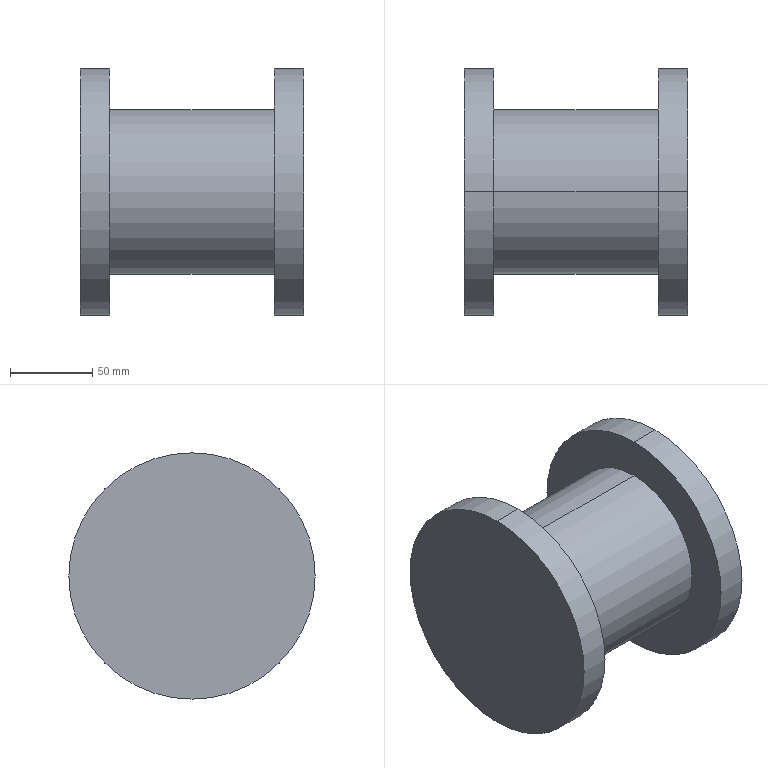Part | SolidWorks | features ICE 2, Extrusion 1 | 1 solid | 10 faces | box 136 x 150 x 150 mm | volume 1421571 mm3 | cylinder 6 | plane 4 | commonest cylinder face diameters 150 x4 100 x2
STEP:
#1=CARTESIAN_POINT('',(-118.,0.,-75.));
#2=VERTEX_POINT('',#1);
#3=CARTESIAN_POINT('',(-118.,0.,75.));
#4=VERTEX_POINT('',#3);
#5=CARTESIAN_POINT('',(-118.,0.,0.));
#6=DIRECTION('',(1.,0.,0.));
#7=DIRECTION('',(0.,0.,-1.));
#8=AXIS2_PLACEMENT_3D('',#5,#6,#7);
#9=CIRCLE('',#8,75.);
#10=EDGE_CURVE('',#2,#4,#9,.T.);
#11=ORIENTED_EDGE('',*,*,#10,.T.);
#12=CARTESIAN_POINT('',(-100.,0.,75.));
#13=VERTEX_POINT('',#12);
#14=CARTESIAN_POINT('',(-118.,0.,75.));
#15=DIRECTION('',(1.,0.,0.));
#16=VECTOR('',#15,1000.);
#17=LINE('',#14,#16);
#18=EDGE_CURVE('',#4,#13,#17,.T.);
#19=ORIENTED_EDGE('',*,*,#18,.T.);
#20=CARTESIAN_POINT('',(-100.,0.,-75.));
#21=VERTEX_POINT('',#20);
#22=CARTESIAN_POINT('',(-100.,0.,0.));
#23=DIRECTION('',(1.,0.,0.));
#24=DIRECTION('',(0.,0.,-1.));
#25=AXIS2_PLACEMENT_3D('',#22,#23,#24);
#26=CIRCLE('',#25,75.);
#27=EDGE_CURVE('',#21,#13,#26,.T.);
#28=ORIENTED_EDGE('',*,*,#27,.F.);
#29=CARTESIAN_POINT('',(-118.,0.,-75.));
#30=DIRECTION('',(1.,0.,0.));
#31=VECTOR('',#30,1000.);
#32=LINE('',#29,#31);
#33=EDGE_CURVE('',#2,#21,#32,.T.);
#34=ORIENTED_EDGE('',*,*,#33,.F.);
#35=EDGE_LOOP('',(#11,#19,#28,#34));
#36=FACE_OUTER_BOUND('',#35,.T.);
#37=CARTESIAN_POINT('',(-118.,0.,0.));
#38=DIRECTION('',(1.,0.,0.));
#39=DIRECTION('',(0.,0.,-1.));
#40=AXIS2_PLACEMENT_3D('',#37,#38,#39);
#41=CYLINDRICAL_SURFACE('',#40,75.);
#42=ADVANCED_FACE('',(#36),#41,.T.);
#43=CARTESIAN_POINT('',(-100.,0.,-50.));
#44=VERTEX_POINT('',#43);
#45=CARTESIAN_POINT('',(-100.,0.,50.));
#46=VERTEX_POINT('',#45);
#47=CARTESIAN_POINT('',(-100.,0.,0.));
#48=DIRECTION('',(1.,0.,0.));
#49=DIRECTION('',(0.,0.,-1.));
#50=AXIS2_PLACEMENT_3D('',#47,#48,#49);
#51=CIRCLE('',#50,50.);
#52=EDGE_CURVE('',#44,#46,#51,.T.);
#53=ORIENTED_EDGE('',*,*,#52,.T.);
#54=CARTESIAN_POINT('',(0.,0.,50.));
#55=VERTEX_POINT('',#54);
#56=CARTESIAN_POINT('',(-100.,0.,50.));
#57=DIRECTION('',(1.,0.,0.));
#58=VECTOR('',#57,1000.);
#59=LINE('',#56,#58);
#60=EDGE_CURVE('',#46,#55,#59,.T.);
#61=ORIENTED_EDGE('',*,*,#60,.T.);
#62=CARTESIAN_POINT('',(0.,0.,-50.));
#63=VERTEX_POINT('',#62);
#64=CARTESIAN_POINT('',(0.,0.,0.));
#65=DIRECTION('',(1.,0.,0.));
#66=DIRECTION('',(0.,0.,-1.));
#67=AXIS2_PLACEMENT_3D('',#64,#65,#66);
#68=CIRCLE('',#67,50.);
#69=EDGE_CURVE('',#63,#55,#68,.T.);
#70=ORIENTED_EDGE('',*,*,#69,.F.);
#71=CARTESIAN_POINT('',(-100.,0.,-50.));
#72=DIRECTION('',(1.,0.,0.));
#73=VECTOR('',#72,1000.);
#74=LINE('',#71,#73);
#75=EDGE_CURVE('',#44,#63,#74,.T.);
#76=ORIENTED_EDGE('',*,*,#75,.F.);
#77=EDGE_LOOP('',(#53,#61,#70,#76));
#78=FACE_OUTER_BOUND('',#77,.T.);
#79=CARTESIAN_POINT('',(-100.,0.,0.));
#80=DIRECTION('',(1.,0.,0.));
#81=DIRECTION('',(0.,0.,-1.));
#82=AXIS2_PLACEMENT_3D('',#79,#80,#81);
#83=CYLINDRICAL_SURFACE('',#82,50.);
#84=ADVANCED_FACE('',(#78),#83,.T.);
#85=CARTESIAN_POINT('',(18.,0.,-75.));
#86=VERTEX_POINT('',#85);
#87=CARTESIAN_POINT('',(18.,0.,75.));
#88=VERTEX_POINT('',#87);
#89=CARTESIAN_POINT('',(18.,0.,0.));
#90=DIRECTION('',(1.,0.,0.));
#91=DIRECTION('',(0.,0.,-1.));
#92=AXIS2_PLACEMENT_3D('',#89,#90,#91);
#93=CIRCLE('',#92,75.);
#94=EDGE_CURVE('',#86,#88,#93,.T.);
#95=ORIENTED_EDGE('',*,*,#94,.F.);
#96=CARTESIAN_POINT('',(0.,0.,-75.));
#97=VERTEX_POINT('',#96);
#98=CARTESIAN_POINT('',(18.,0.,-75.));
#99=DIRECTION('',(-1.,0.,0.));
#100=VECTOR('',#99,1000.);
#101=LINE('',#98,#100);
#102=EDGE_CURVE('',#86,#97,#101,.T.);
#103=ORIENTED_EDGE('',*,*,#102,.T.);
#104=CARTESIAN_POINT('',(0.,0.,75.));
#105=VERTEX_POINT('',#104);
#106=CARTESIAN_POINT('',(0.,0.,0.));
#107=DIRECTION('',(1.,0.,0.));
#108=DIRECTION('',(0.,0.,-1.));
#109=AXIS2_PLACEMENT_3D('',#106,#107,#108);
#110=CIRCLE('',#109,75.);
#111=EDGE_CURVE('',#97,#105,#110,.T.);
#112=ORIENTED_EDGE('',*,*,#111,.T.);
#113=CARTESIAN_POINT('',(18.,0.,75.));
#114=DIRECTION('',(-1.,0.,0.));
#115=VECTOR('',#114,1000.);
#116=LINE('',#113,#115);
#117=EDGE_CURVE('',#88,#105,#116,.T.);
#118=ORIENTED_EDGE('',*,*,#117,.F.);
#119=EDGE_LOOP('',(#95,#103,#112,#118));
#120=FACE_OUTER_BOUND('',#119,.T.);
#121=CARTESIAN_POINT('',(18.,0.,0.));
#122=DIRECTION('',(-1.,0.,0.));
#123=DIRECTION('',(0.,0.,1.));
#124=AXIS2_PLACEMENT_3D('',#121,#122,#123);
#125=CYLINDRICAL_SURFACE('',#124,75.);
#126=ADVANCED_FACE('',(#120),#125,.T.);
#127=ORIENTED_EDGE('',*,*,#102,.F.);
#128=CARTESIAN_POINT('',(18.,0.,0.));
#129=DIRECTION('',(1.,0.,0.));
#130=DIRECTION('',(0.,0.,-1.));
#131=AXIS2_PLACEMENT_3D('',#128,#129,#130);
#132=CIRCLE('',#131,75.);
#133=EDGE_CURVE('',#88,#86,#132,.T.);
#134=ORIENTED_EDGE('',*,*,#133,.F.);
#135=ORIENTED_EDGE('',*,*,#117,.T.);
#136=CARTESIAN_POINT('',(0.,0.,0.));
#137=DIRECTION('',(1.,0.,0.));
#138=DIRECTION('',(0.,0.,-1.));
#139=AXIS2_PLACEMENT_3D('',#136,#137,#138);
#140=CIRCLE('',#139,75.);
#141=EDGE_CURVE('',#105,#97,#140,.T.);
#142=ORIENTED_EDGE('',*,*,#141,.T.);
#143=EDGE_LOOP('',(#127,#134,#135,#142));
#144=FACE_OUTER_BOUND('',#143,.T.);
#145=CARTESIAN_POINT('',(18.,0.,0.));
#146=DIRECTION('',(-1.,0.,0.));
#147=DIRECTION('',(0.,0.,1.));
#148=AXIS2_PLACEMENT_3D('',#145,#146,#147);
#149=CYLINDRICAL_SURFACE('',#148,75.);
#150=ADVANCED_FACE('',(#144),#149,.T.);
#151=ORIENTED_EDGE('',*,*,#69,.T.);
#152=CARTESIAN_POINT('',(0.,0.,0.));
#153=DIRECTION('',(1.,0.,0.));
#154=DIRECTION('',(0.,0.,-1.));
#155=AXIS2_PLACEMENT_3D('',#152,#153,#154);
#156=CIRCLE('',#155,50.);
#157=EDGE_CURVE('',#55,#63,#156,.T.);
#158=ORIENTED_EDGE('',*,*,#157,.T.);
#159=EDGE_LOOP('',(#151,#158));
#160=FACE_BOUND('',#159,.T.);
#161=ORIENTED_EDGE('',*,*,#141,.F.);
#162=ORIENTED_EDGE('',*,*,#111,.F.);
#163=EDGE_LOOP('',(#161,#162));
#164=FACE_OUTER_BOUND('',#163,.T.);
#165=CARTESIAN_POINT('',(0.,0.,0.));
#166=DIRECTION('',(1.,0.,0.));
#167=DIRECTION('',(0.,0.,-1.));
#168=AXIS2_PLACEMENT_3D('',#165,#166,#167);
#169=PLANE('',#168);
#170=ADVANCED_FACE('',(#160,#164),#169,.F.);
#171=ORIENTED_EDGE('',*,*,#133,.T.);
#172=ORIENTED_EDGE('',*,*,#94,.T.);
#173=EDGE_LOOP('',(#171,#172));
#174=FACE_OUTER_BOUND('',#173,.T.);
#175=CARTESIAN_POINT('',(18.,0.,0.));
#176=DIRECTION('',(1.,0.,0.));
#177=DIRECTION('',(0.,0.,-1.));
#178=AXIS2_PLACEMENT_3D('',#175,#176,#177);
#179=PLANE('',#178);
#180=ADVANCED_FACE('',(#174),#179,.T.);
#181=ORIENTED_EDGE('',*,*,#60,.F.);
#182=CARTESIAN_POINT('',(-100.,0.,0.));
#183=DIRECTION('',(1.,0.,0.));
#184=DIRECTION('',(0.,0.,-1.));
#185=AXIS2_PLACEMENT_3D('',#182,#183,#184);
#186=CIRCLE('',#185,50.);
#187=EDGE_CURVE('',#46,#44,#186,.T.);
#188=ORIENTED_EDGE('',*,*,#187,.T.);
#189=ORIENTED_EDGE('',*,*,#75,.T.);
#190=ORIENTED_EDGE('',*,*,#157,.F.);
#191=EDGE_LOOP('',(#181,#188,#189,#190));
#192=FACE_OUTER_BOUND('',#191,.T.);
#193=CARTESIAN_POINT('',(-100.,0.,0.));
#194=DIRECTION('',(1.,0.,0.));
#195=DIRECTION('',(0.,0.,-1.));
#196=AXIS2_PLACEMENT_3D('',#193,#194,#195);
#197=CYLINDRICAL_SURFACE('',#196,50.);
#198=ADVANCED_FACE('',(#192),#197,.T.);
#199=ORIENTED_EDGE('',*,*,#18,.F.);
#200=CARTESIAN_POINT('',(-118.,0.,0.));
#201=DIRECTION('',(1.,0.,0.));
#202=DIRECTION('',(0.,0.,-1.));
#203=AXIS2_PLACEMENT_3D('',#200,#201,#202);
#204=CIRCLE('',#203,75.);
#205=EDGE_CURVE('',#4,#2,#204,.T.);
#206=ORIENTED_EDGE('',*,*,#205,.T.);
#207=ORIENTED_EDGE('',*,*,#33,.T.);
#208=CARTESIAN_POINT('',(-100.,0.,0.));
#209=DIRECTION('',(1.,0.,0.));
#210=DIRECTION('',(0.,0.,-1.));
#211=AXIS2_PLACEMENT_3D('',#208,#209,#210);
#212=CIRCLE('',#211,75.);
#213=EDGE_CURVE('',#13,#21,#212,.T.);
#214=ORIENTED_EDGE('',*,*,#213,.F.);
#215=EDGE_LOOP('',(#199,#206,#207,#214));
#216=FACE_OUTER_BOUND('',#215,.T.);
#217=CARTESIAN_POINT('',(-118.,0.,0.));
#218=DIRECTION('',(1.,0.,0.));
#219=DIRECTION('',(0.,0.,-1.));
#220=AXIS2_PLACEMENT_3D('',#217,#218,#219);
#221=CYLINDRICAL_SURFACE('',#220,75.);
#222=ADVANCED_FACE('',(#216),#221,.T.);
#223=ORIENTED_EDGE('',*,*,#10,.F.);
#224=ORIENTED_EDGE('',*,*,#205,.F.);
#225=EDGE_LOOP('',(#223,#224));
#226=FACE_OUTER_BOUND('',#225,.T.);
#227=CARTESIAN_POINT('',(-118.,0.,0.));
#228=DIRECTION('',(1.,0.,0.));
#229=DIRECTION('',(0.,0.,-1.));
#230=AXIS2_PLACEMENT_3D('',#227,#228,#229);
#231=PLANE('',#230);
#232=ADVANCED_FACE('',(#226),#231,.F.);
#233=ORIENTED_EDGE('',*,*,#52,.F.);
#234=ORIENTED_EDGE('',*,*,#187,.F.);
#235=EDGE_LOOP('',(#233,#234));
#236=FACE_BOUND('',#235,.T.);
#237=ORIENTED_EDGE('',*,*,#27,.T.);
#238=ORIENTED_EDGE('',*,*,#213,.T.);
#239=EDGE_LOOP('',(#237,#238));
#240=FACE_OUTER_BOUND('',#239,.T.);
#241=CARTESIAN_POINT('',(-100.,0.,0.));
#242=DIRECTION('',(1.,0.,0.));
#243=DIRECTION('',(0.,0.,-1.));
#244=AXIS2_PLACEMENT_3D('',#241,#242,#243);
#245=PLANE('',#244);
#246=ADVANCED_FACE('',(#236,#240),#245,.T.);
#247=CLOSED_SHELL('',(#42,#84,#126,#150,#170,#180,#198,#222,#232,#246));
#248=MANIFOLD_SOLID_BREP('',#247);
#249=CARTESIAN_POINT('',(0.,0.,0.));
#250=DIRECTION('',(0.,0.,1.));
#251=DIRECTION('',(1.,0.,0.));
#252=AXIS2_PLACEMENT_3D('',#249,#250,#251);
#253=(LENGTH_UNIT()NAMED_UNIT(*)SI_UNIT(.MILLI.,.METRE.));
#254=UNCERTAINTY_MEASURE_WITH_UNIT(LENGTH_MEASURE(0.00001),#253,'','');
#255=(NAMED_UNIT(*)PLANE_ANGLE_UNIT()SI_UNIT($,.RADIAN.));
#256=(NAMED_UNIT(*)SI_UNIT($,.STERADIAN.)SOLID_ANGLE_UNIT());
#257=(GEOMETRIC_REPRESENTATION_CONTEXT(3)GLOBAL_UNCERTAINTY_ASSIGNED_CONTEXT((#254))GLOBAL_UNIT_ASSIGNED_CONTEXT((#253,#255,#256))REPRESENTATION_CONTEXT('',''));
#258=ADVANCED_BREP_SHAPE_REPRESENTATION('',(#248,#252),#257);